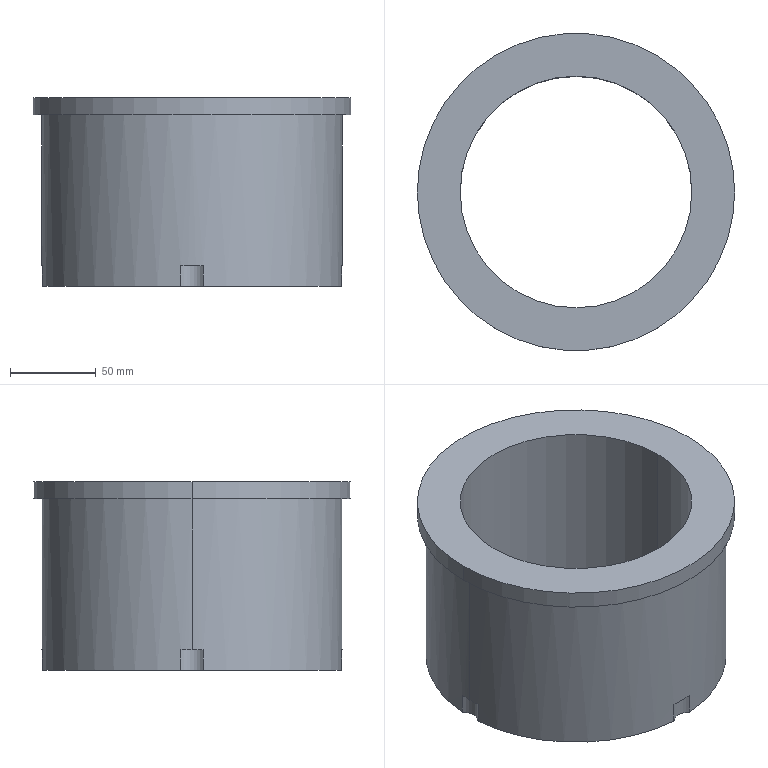Part | SolidWorks | features ICE 5, HoleWzd 1, Revolution 1 | 1 solid | 18 faces | box 185 x 185 x 110 mm | volume 1098272 mm3 | cylinder 11 | plane 7 | commonest cylinder face diameters 18 x5 135 x2 175 x2 185 x2
STEP:
#1=CARTESIAN_POINT('',(453.731,234.744,-1357.693));
#2=VERTEX_POINT('',#1);
#3=CARTESIAN_POINT('',(588.731,234.744,-1357.693));
#4=VERTEX_POINT('',#3);
#5=CARTESIAN_POINT('',(521.231,234.744,-1357.693));
#6=DIRECTION('',(0.,0.,1.));
#7=DIRECTION('',(1.,0.,0.));
#8=AXIS2_PLACEMENT_3D('',#5,#6,#7);
#9=CIRCLE('',#8,67.5);
#10=EDGE_CURVE('',#2,#4,#9,.T.);
#11=ORIENTED_EDGE('',*,*,#10,.F.);
#12=CARTESIAN_POINT('',(453.731,234.744,-1247.693));
#13=VERTEX_POINT('',#12);
#14=CARTESIAN_POINT('',(453.731,234.744,-1247.693));
#15=DIRECTION('',(0.,0.,1.));
#16=VECTOR('',#15,1000.);
#17=LINE('',#14,#16);
#18=EDGE_CURVE('',#2,#13,#17,.T.);
#19=ORIENTED_EDGE('',*,*,#18,.T.);
#20=CARTESIAN_POINT('',(588.731,234.744,-1247.693));
#21=VERTEX_POINT('',#20);
#22=CARTESIAN_POINT('',(521.231,234.744,-1247.693));
#23=DIRECTION('',(0.,0.,1.));
#24=DIRECTION('',(1.,0.,0.));
#25=AXIS2_PLACEMENT_3D('',#22,#23,#24);
#26=CIRCLE('',#25,67.5);
#27=EDGE_CURVE('',#13,#21,#26,.T.);
#28=ORIENTED_EDGE('',*,*,#27,.T.);
#29=CARTESIAN_POINT('',(588.731,234.744,-1247.693));
#30=DIRECTION('',(0.,0.,1.));
#31=VECTOR('',#30,1000.);
#32=LINE('',#29,#31);
#33=EDGE_CURVE('',#4,#21,#32,.T.);
#34=ORIENTED_EDGE('',*,*,#33,.F.);
#35=EDGE_LOOP('',(#11,#19,#28,#34));
#36=FACE_OUTER_BOUND('',#35,.T.);
#37=CARTESIAN_POINT('',(521.231,234.744,-1247.693));
#38=DIRECTION('',(0.,0.,1.));
#39=DIRECTION('',(1.,0.,0.));
#40=AXIS2_PLACEMENT_3D('',#37,#38,#39);
#41=CYLINDRICAL_SURFACE('',#40,67.5);
#42=ADVANCED_FACE('',(#36),#41,.F.);
#43=CARTESIAN_POINT('',(605.731,234.744,-1345.693));
#44=VERTEX_POINT('',#43);
#45=CARTESIAN_POINT('',(608.49,241.229,-1345.693));
#46=VERTEX_POINT('',#45);
#47=CARTESIAN_POINT('',(614.731,234.744,-1345.693));
#48=DIRECTION('',(0.,0.,-1.));
#49=DIRECTION('',(-1.,0.,0.));
#50=AXIS2_PLACEMENT_3D('',#47,#48,#49);
#51=CIRCLE('',#50,9.);
#52=EDGE_CURVE('',#44,#46,#51,.T.);
#53=ORIENTED_EDGE('',*,*,#52,.F.);
#54=CARTESIAN_POINT('',(605.731,234.744,-1357.693));
#55=VERTEX_POINT('',#54);
#56=CARTESIAN_POINT('',(605.731,234.744,-1345.693));
#57=DIRECTION('',(0.,0.,-1.));
#58=VECTOR('',#57,1000.);
#59=LINE('',#56,#58);
#60=EDGE_CURVE('',#44,#55,#59,.T.);
#61=ORIENTED_EDGE('',*,*,#60,.T.);
#62=CARTESIAN_POINT('',(608.49,241.229,-1357.693));
#63=VERTEX_POINT('',#62);
#64=CARTESIAN_POINT('',(614.731,234.744,-1357.693));
#65=DIRECTION('',(0.,0.,-1.));
#66=DIRECTION('',(-1.,0.,0.));
#67=AXIS2_PLACEMENT_3D('',#64,#65,#66);
#68=CIRCLE('',#67,9.);
#69=EDGE_CURVE('',#55,#63,#68,.T.);
#70=ORIENTED_EDGE('',*,*,#69,.T.);
#71=CARTESIAN_POINT('',(608.49,241.229,-1345.693));
#72=DIRECTION('',(0.,0.,-1.));
#73=VECTOR('',#72,1000.);
#74=LINE('',#71,#73);
#75=EDGE_CURVE('',#46,#63,#74,.T.);
#76=ORIENTED_EDGE('',*,*,#75,.F.);
#77=EDGE_LOOP('',(#53,#61,#70,#76));
#78=FACE_OUTER_BOUND('',#77,.T.);
#79=CARTESIAN_POINT('',(614.731,234.744,-1345.693));
#80=DIRECTION('',(0.,0.,-1.));
#81=DIRECTION('',(-1.,0.,0.));
#82=AXIS2_PLACEMENT_3D('',#79,#80,#81);
#83=CYLINDRICAL_SURFACE('',#82,9.);
#84=ADVANCED_FACE('',(#78),#83,.F.);
#85=CARTESIAN_POINT('',(433.731,234.744,-1345.693));
#86=VERTEX_POINT('',#85);
#87=CARTESIAN_POINT('',(433.971,241.229,-1345.693));
#88=VERTEX_POINT('',#87);
#89=CARTESIAN_POINT('',(521.231,234.744,-1345.693));
#90=DIRECTION('',(0.,0.,-1.));
#91=DIRECTION('',(-1.,0.,0.));
#92=AXIS2_PLACEMENT_3D('',#89,#90,#91);
#93=CIRCLE('',#92,87.5);
#94=EDGE_CURVE('',#86,#88,#93,.T.);
#95=ORIENTED_EDGE('',*,*,#94,.F.);
#96=CARTESIAN_POINT('',(433.731,234.744,-1257.693));
#97=VERTEX_POINT('',#96);
#98=CARTESIAN_POINT('',(433.731,234.744,-1357.693));
#99=DIRECTION('',(0.,0.,1.));
#100=VECTOR('',#99,1000.);
#101=LINE('',#98,#100);
#102=EDGE_CURVE('',#86,#97,#101,.T.);
#103=ORIENTED_EDGE('',*,*,#102,.T.);
#104=CARTESIAN_POINT('',(608.731,234.744,-1257.693));
#105=VERTEX_POINT('',#104);
#106=CARTESIAN_POINT('',(521.231,234.744,-1257.693));
#107=DIRECTION('',(0.,0.,-1.));
#108=DIRECTION('',(-1.,0.,0.));
#109=AXIS2_PLACEMENT_3D('',#106,#107,#108);
#110=CIRCLE('',#109,87.5);
#111=EDGE_CURVE('',#97,#105,#110,.T.);
#112=ORIENTED_EDGE('',*,*,#111,.T.);
#113=CARTESIAN_POINT('',(608.731,234.744,-1345.693));
#114=VERTEX_POINT('',#113);
#115=CARTESIAN_POINT('',(608.731,234.744,-1357.693));
#116=DIRECTION('',(0.,0.,1.));
#117=VECTOR('',#116,1000.);
#118=LINE('',#115,#117);
#119=EDGE_CURVE('',#114,#105,#118,.T.);
#120=ORIENTED_EDGE('',*,*,#119,.F.);
#121=CARTESIAN_POINT('',(521.231,234.744,-1345.693));
#122=DIRECTION('',(0.,0.,-1.));
#123=DIRECTION('',(-1.,0.,0.));
#124=AXIS2_PLACEMENT_3D('',#121,#122,#123);
#125=CIRCLE('',#124,87.5);
#126=EDGE_CURVE('',#46,#114,#125,.T.);
#127=ORIENTED_EDGE('',*,*,#126,.F.);
#128=ORIENTED_EDGE('',*,*,#75,.T.);
#129=CARTESIAN_POINT('',(527.716,322.003,-1357.693));
#130=VERTEX_POINT('',#129);
#131=CARTESIAN_POINT('',(521.231,234.744,-1357.693));
#132=DIRECTION('',(0.,0.,-1.));
#133=DIRECTION('',(-1.,0.,0.));
#134=AXIS2_PLACEMENT_3D('',#131,#132,#133);
#135=CIRCLE('',#134,87.5);
#136=EDGE_CURVE('',#130,#63,#135,.T.);
#137=ORIENTED_EDGE('',*,*,#136,.F.);
#138=CARTESIAN_POINT('',(527.716,322.003,-1345.693));
#139=VERTEX_POINT('',#138);
#140=CARTESIAN_POINT('',(527.716,322.003,-1345.693));
#141=DIRECTION('',(0.,0.,-1.));
#142=VECTOR('',#141,1000.);
#143=LINE('',#140,#142);
#144=EDGE_CURVE('',#139,#130,#143,.T.);
#145=ORIENTED_EDGE('',*,*,#144,.F.);
#146=CARTESIAN_POINT('',(514.746,322.003,-1345.693));
#147=VERTEX_POINT('',#146);
#148=CARTESIAN_POINT('',(521.231,234.744,-1345.693));
#149=DIRECTION('',(0.,0.,-1.));
#150=DIRECTION('',(-1.,0.,0.));
#151=AXIS2_PLACEMENT_3D('',#148,#149,#150);
#152=CIRCLE('',#151,87.5);
#153=EDGE_CURVE('',#147,#139,#152,.T.);
#154=ORIENTED_EDGE('',*,*,#153,.F.);
#155=CARTESIAN_POINT('',(514.746,322.003,-1357.693));
#156=VERTEX_POINT('',#155);
#157=CARTESIAN_POINT('',(514.746,322.003,-1345.693));
#158=DIRECTION('',(0.,0.,-1.));
#159=VECTOR('',#158,1000.);
#160=LINE('',#157,#159);
#161=EDGE_CURVE('',#147,#156,#160,.T.);
#162=ORIENTED_EDGE('',*,*,#161,.T.);
#163=CARTESIAN_POINT('',(433.971,241.229,-1357.693));
#164=VERTEX_POINT('',#163);
#165=CARTESIAN_POINT('',(521.231,234.744,-1357.693));
#166=DIRECTION('',(0.,0.,-1.));
#167=DIRECTION('',(-1.,0.,0.));
#168=AXIS2_PLACEMENT_3D('',#165,#166,#167);
#169=CIRCLE('',#168,87.5);
#170=EDGE_CURVE('',#164,#156,#169,.T.);
#171=ORIENTED_EDGE('',*,*,#170,.F.);
#172=CARTESIAN_POINT('',(433.971,241.229,-1345.693));
#173=DIRECTION('',(0.,0.,-1.));
#174=VECTOR('',#173,1000.);
#175=LINE('',#172,#174);
#176=EDGE_CURVE('',#88,#164,#175,.T.);
#177=ORIENTED_EDGE('',*,*,#176,.F.);
#178=EDGE_LOOP('',(#95,#103,#112,#120,#127,#128,#137,#145,#154,#162,#171,#177));
#179=FACE_OUTER_BOUND('',#178,.T.);
#180=CARTESIAN_POINT('',(521.231,234.744,-1357.693));
#181=DIRECTION('',(0.,0.,1.));
#182=DIRECTION('',(1.,0.,0.));
#183=AXIS2_PLACEMENT_3D('',#180,#181,#182);
#184=CYLINDRICAL_SURFACE('',#183,87.5);
#185=ADVANCED_FACE('',(#179),#184,.T.);
#186=CARTESIAN_POINT('',(613.731,234.744,-1257.693));
#187=VERTEX_POINT('',#186);
#188=CARTESIAN_POINT('',(428.731,234.744,-1257.693));
#189=VERTEX_POINT('',#188);
#190=CARTESIAN_POINT('',(521.231,234.744,-1257.693));
#191=DIRECTION('',(0.,0.,1.));
#192=DIRECTION('',(1.,0.,0.));
#193=AXIS2_PLACEMENT_3D('',#190,#191,#192);
#194=CIRCLE('',#193,92.5);
#195=EDGE_CURVE('',#187,#189,#194,.T.);
#196=ORIENTED_EDGE('',*,*,#195,.T.);
#197=CARTESIAN_POINT('',(428.731,234.744,-1247.693));
#198=VERTEX_POINT('',#197);
#199=CARTESIAN_POINT('',(428.731,234.744,-1257.693));
#200=DIRECTION('',(0.,0.,1.));
#201=VECTOR('',#200,1000.);
#202=LINE('',#199,#201);
#203=EDGE_CURVE('',#189,#198,#202,.T.);
#204=ORIENTED_EDGE('',*,*,#203,.T.);
#205=CARTESIAN_POINT('',(613.731,234.744,-1247.693));
#206=VERTEX_POINT('',#205);
#207=CARTESIAN_POINT('',(521.231,234.744,-1247.693));
#208=DIRECTION('',(0.,0.,1.));
#209=DIRECTION('',(1.,0.,0.));
#210=AXIS2_PLACEMENT_3D('',#207,#208,#209);
#211=CIRCLE('',#210,92.5);
#212=EDGE_CURVE('',#206,#198,#211,.T.);
#213=ORIENTED_EDGE('',*,*,#212,.F.);
#214=CARTESIAN_POINT('',(613.731,234.744,-1257.693));
#215=DIRECTION('',(0.,0.,1.));
#216=VECTOR('',#215,1000.);
#217=LINE('',#214,#216);
#218=EDGE_CURVE('',#187,#206,#217,.T.);
#219=ORIENTED_EDGE('',*,*,#218,.F.);
#220=EDGE_LOOP('',(#196,#204,#213,#219));
#221=FACE_OUTER_BOUND('',#220,.T.);
#222=CARTESIAN_POINT('',(521.231,234.744,-1257.693));
#223=DIRECTION('',(0.,0.,1.));
#224=DIRECTION('',(1.,0.,0.));
#225=AXIS2_PLACEMENT_3D('',#222,#223,#224);
#226=CYLINDRICAL_SURFACE('',#225,92.5);
#227=ADVANCED_FACE('',(#221),#226,.T.);
#228=CARTESIAN_POINT('',(608.49,228.259,-1357.693));
#229=VERTEX_POINT('',#228);
#230=CARTESIAN_POINT('',(614.731,234.744,-1357.693));
#231=DIRECTION('',(0.,0.,-1.));
#232=DIRECTION('',(-1.,0.,0.));
#233=AXIS2_PLACEMENT_3D('',#230,#231,#232);
#234=CIRCLE('',#233,9.);
#235=EDGE_CURVE('',#229,#55,#234,.T.);
#236=ORIENTED_EDGE('',*,*,#235,.F.);
#237=CARTESIAN_POINT('',(527.716,147.485,-1357.693));
#238=VERTEX_POINT('',#237);
#239=CARTESIAN_POINT('',(521.231,234.744,-1357.693));
#240=DIRECTION('',(0.,0.,-1.));
#241=DIRECTION('',(-1.,0.,0.));
#242=AXIS2_PLACEMENT_3D('',#239,#240,#241);
#243=CIRCLE('',#242,87.5);
#244=EDGE_CURVE('',#229,#238,#243,.T.);
#245=ORIENTED_EDGE('',*,*,#244,.T.);
#246=CARTESIAN_POINT('',(514.746,147.485,-1357.693));
#247=VERTEX_POINT('',#246);
#248=CARTESIAN_POINT('',(521.231,141.244,-1357.693));
#249=DIRECTION('',(0.,0.,-1.));
#250=DIRECTION('',(-1.,0.,0.));
#251=AXIS2_PLACEMENT_3D('',#248,#249,#250);
#252=CIRCLE('',#251,9.);
#253=EDGE_CURVE('',#247,#238,#252,.T.);
#254=ORIENTED_EDGE('',*,*,#253,.F.);
#255=CARTESIAN_POINT('',(433.971,228.259,-1357.693));
#256=VERTEX_POINT('',#255);
#257=CARTESIAN_POINT('',(521.231,234.744,-1357.693));
#258=DIRECTION('',(0.,0.,-1.));
#259=DIRECTION('',(-1.,0.,0.));
#260=AXIS2_PLACEMENT_3D('',#257,#258,#259);
#261=CIRCLE('',#260,87.5);
#262=EDGE_CURVE('',#247,#256,#261,.T.);
#263=ORIENTED_EDGE('',*,*,#262,.T.);
#264=CARTESIAN_POINT('',(427.731,234.744,-1357.693));
#265=DIRECTION('',(0.,0.,-1.));
#266=DIRECTION('',(-1.,0.,0.));
#267=AXIS2_PLACEMENT_3D('',#264,#265,#266);
#268=CIRCLE('',#267,9.);
#269=EDGE_CURVE('',#164,#256,#268,.T.);
#270=ORIENTED_EDGE('',*,*,#269,.F.);
#271=ORIENTED_EDGE('',*,*,#170,.T.);
#272=CARTESIAN_POINT('',(521.231,328.244,-1357.693));
#273=DIRECTION('',(0.,0.,-1.));
#274=DIRECTION('',(-1.,0.,0.));
#275=AXIS2_PLACEMENT_3D('',#272,#273,#274);
#276=CIRCLE('',#275,9.);
#277=EDGE_CURVE('',#130,#156,#276,.T.);
#278=ORIENTED_EDGE('',*,*,#277,.F.);
#279=ORIENTED_EDGE('',*,*,#136,.T.);
#280=ORIENTED_EDGE('',*,*,#69,.F.);
#281=EDGE_LOOP('',(#236,#245,#254,#263,#270,#271,#278,#279,#280));
#282=FACE_OUTER_BOUND('',#281,.T.);
#283=CARTESIAN_POINT('',(521.231,234.744,-1357.693));
#284=DIRECTION('',(0.,0.,1.));
#285=DIRECTION('',(1.,0.,0.));
#286=AXIS2_PLACEMENT_3D('',#283,#284,#285);
#287=CIRCLE('',#286,67.5);
#288=EDGE_CURVE('',#4,#2,#287,.T.);
#289=ORIENTED_EDGE('',*,*,#288,.T.);
#290=ORIENTED_EDGE('',*,*,#10,.T.);
#291=EDGE_LOOP('',(#289,#290));
#292=FACE_BOUND('',#291,.T.);
#293=CARTESIAN_POINT('',(521.231,234.744,-1357.693));
#294=DIRECTION('',(0.,0.,-1.));
#295=DIRECTION('',(-1.,0.,0.));
#296=AXIS2_PLACEMENT_3D('',#293,#294,#295);
#297=PLANE('',#296);
#298=ADVANCED_FACE('',(#282,#292),#297,.T.);
#299=ORIENTED_EDGE('',*,*,#203,.F.);
#300=CARTESIAN_POINT('',(521.231,234.744,-1257.693));
#301=DIRECTION('',(0.,0.,1.));
#302=DIRECTION('',(1.,0.,0.));
#303=AXIS2_PLACEMENT_3D('',#300,#301,#302);
#304=CIRCLE('',#303,92.5);
#305=EDGE_CURVE('',#189,#187,#304,.T.);
#306=ORIENTED_EDGE('',*,*,#305,.T.);
#307=ORIENTED_EDGE('',*,*,#218,.T.);
#308=CARTESIAN_POINT('',(521.231,234.744,-1247.693));
#309=DIRECTION('',(0.,0.,1.));
#310=DIRECTION('',(1.,0.,0.));
#311=AXIS2_PLACEMENT_3D('',#308,#309,#310);
#312=CIRCLE('',#311,92.5);
#313=EDGE_CURVE('',#198,#206,#312,.T.);
#314=ORIENTED_EDGE('',*,*,#313,.F.);
#315=EDGE_LOOP('',(#299,#306,#307,#314));
#316=FACE_OUTER_BOUND('',#315,.T.);
#317=CARTESIAN_POINT('',(521.231,234.744,-1257.693));
#318=DIRECTION('',(0.,0.,1.));
#319=DIRECTION('',(1.,0.,0.));
#320=AXIS2_PLACEMENT_3D('',#317,#318,#319);
#321=CYLINDRICAL_SURFACE('',#320,92.5);
#322=ADVANCED_FACE('',(#316),#321,.T.);
#323=CARTESIAN_POINT('',(521.231,234.744,-1257.693));
#324=DIRECTION('',(0.,0.,-1.));
#325=DIRECTION('',(-1.,0.,0.));
#326=AXIS2_PLACEMENT_3D('',#323,#324,#325);
#327=CIRCLE('',#326,87.5);
#328=EDGE_CURVE('',#105,#97,#327,.T.);
#329=ORIENTED_EDGE('',*,*,#328,.F.);
#330=ORIENTED_EDGE('',*,*,#111,.F.);
#331=EDGE_LOOP('',(#329,#330));
#332=FACE_BOUND('',#331,.T.);
#333=ORIENTED_EDGE('',*,*,#195,.F.);
#334=ORIENTED_EDGE('',*,*,#305,.F.);
#335=EDGE_LOOP('',(#333,#334));
#336=FACE_OUTER_BOUND('',#335,.T.);
#337=CARTESIAN_POINT('',(613.731,234.744,-1257.693));
#338=DIRECTION('',(0.,0.,-1.));
#339=DIRECTION('',(-1.,0.,0.));
#340=AXIS2_PLACEMENT_3D('',#337,#338,#339);
#341=PLANE('',#340);
#342=ADVANCED_FACE('',(#332,#336),#341,.T.);
#343=CARTESIAN_POINT('',(521.231,234.744,-1247.693));
#344=DIRECTION('',(0.,0.,1.));
#345=DIRECTION('',(1.,0.,0.));
#346=AXIS2_PLACEMENT_3D('',#343,#344,#345);
#347=CIRCLE('',#346,67.5);
#348=EDGE_CURVE('',#21,#13,#347,.T.);
#349=ORIENTED_EDGE('',*,*,#348,.F.);
#350=ORIENTED_EDGE('',*,*,#27,.F.);
#351=EDGE_LOOP('',(#349,#350));
#352=FACE_BOUND('',#351,.T.);
#353=ORIENTED_EDGE('',*,*,#212,.T.);
#354=ORIENTED_EDGE('',*,*,#313,.T.);
#355=EDGE_LOOP('',(#353,#354));
#356=FACE_OUTER_BOUND('',#355,.T.);
#357=CARTESIAN_POINT('',(521.231,234.744,-1247.693));
#358=DIRECTION('',(0.,0.,1.));
#359=DIRECTION('',(1.,0.,0.));
#360=AXIS2_PLACEMENT_3D('',#357,#358,#359);
#361=PLANE('',#360);
#362=ADVANCED_FACE('',(#352,#356),#361,.T.);
#363=ORIENTED_EDGE('',*,*,#102,.F.);
#364=CARTESIAN_POINT('',(433.971,228.259,-1345.693));
#365=VERTEX_POINT('',#364);
#366=CARTESIAN_POINT('',(521.231,234.744,-1345.693));
#367=DIRECTION('',(0.,0.,-1.));
#368=DIRECTION('',(-1.,0.,0.));
#369=AXIS2_PLACEMENT_3D('',#366,#367,#368);
#370=CIRCLE('',#369,87.5);
#371=EDGE_CURVE('',#365,#86,#370,.T.);
#372=ORIENTED_EDGE('',*,*,#371,.F.);
#373=CARTESIAN_POINT('',(433.971,228.259,-1345.693));
#374=DIRECTION('',(0.,0.,-1.));
#375=VECTOR('',#374,1000.);
#376=LINE('',#373,#375);
#377=EDGE_CURVE('',#365,#256,#376,.T.);
#378=ORIENTED_EDGE('',*,*,#377,.T.);
#379=ORIENTED_EDGE('',*,*,#262,.F.);
#380=CARTESIAN_POINT('',(514.746,147.485,-1345.693));
#381=VERTEX_POINT('',#380);
#382=CARTESIAN_POINT('',(514.746,147.485,-1345.693));
#383=DIRECTION('',(0.,0.,-1.));
#384=VECTOR('',#383,1000.);
#385=LINE('',#382,#384);
#386=EDGE_CURVE('',#381,#247,#385,.T.);
#387=ORIENTED_EDGE('',*,*,#386,.F.);
#388=CARTESIAN_POINT('',(527.716,147.485,-1345.693));
#389=VERTEX_POINT('',#388);
#390=CARTESIAN_POINT('',(521.231,234.744,-1345.693));
#391=DIRECTION('',(0.,0.,-1.));
#392=DIRECTION('',(-1.,0.,0.));
#393=AXIS2_PLACEMENT_3D('',#390,#391,#392);
#394=CIRCLE('',#393,87.5);
#395=EDGE_CURVE('',#389,#381,#394,.T.);
#396=ORIENTED_EDGE('',*,*,#395,.F.);
#397=CARTESIAN_POINT('',(527.716,147.485,-1345.693));
#398=DIRECTION('',(0.,0.,-1.));
#399=VECTOR('',#398,1000.);
#400=LINE('',#397,#399);
#401=EDGE_CURVE('',#389,#238,#400,.T.);
#402=ORIENTED_EDGE('',*,*,#401,.T.);
#403=ORIENTED_EDGE('',*,*,#244,.F.);
#404=CARTESIAN_POINT('',(608.49,228.259,-1345.693));
#405=VERTEX_POINT('',#404);
#406=CARTESIAN_POINT('',(608.49,228.259,-1345.693));
#407=DIRECTION('',(0.,0.,-1.));
#408=VECTOR('',#407,1000.);
#409=LINE('',#406,#408);
#410=EDGE_CURVE('',#405,#229,#409,.T.);
#411=ORIENTED_EDGE('',*,*,#410,.F.);
#412=CARTESIAN_POINT('',(521.231,234.744,-1345.693));
#413=DIRECTION('',(0.,0.,-1.));
#414=DIRECTION('',(-1.,0.,0.));
#415=AXIS2_PLACEMENT_3D('',#412,#413,#414);
#416=CIRCLE('',#415,87.5);
#417=EDGE_CURVE('',#114,#405,#416,.T.);
#418=ORIENTED_EDGE('',*,*,#417,.F.);
#419=ORIENTED_EDGE('',*,*,#119,.T.);
#420=ORIENTED_EDGE('',*,*,#328,.T.);
#421=EDGE_LOOP('',(#363,#372,#378,#379,#387,#396,#402,#403,#411,#418,#419,#420));
#422=FACE_OUTER_BOUND('',#421,.T.);
#423=CARTESIAN_POINT('',(521.231,234.744,-1357.693));
#424=DIRECTION('',(0.,0.,1.));
#425=DIRECTION('',(1.,0.,0.));
#426=AXIS2_PLACEMENT_3D('',#423,#424,#425);
#427=CYLINDRICAL_SURFACE('',#426,87.5);
#428=ADVANCED_FACE('',(#422),#427,.T.);
#429=ORIENTED_EDGE('',*,*,#269,.T.);
#430=ORIENTED_EDGE('',*,*,#377,.F.);
#431=CARTESIAN_POINT('',(427.731,234.744,-1345.693));
#432=DIRECTION('',(0.,0.,-1.));
#433=DIRECTION('',(-1.,0.,0.));
#434=AXIS2_PLACEMENT_3D('',#431,#432,#433);
#435=CIRCLE('',#434,9.);
#436=EDGE_CURVE('',#88,#365,#435,.T.);
#437=ORIENTED_EDGE('',*,*,#436,.F.);
#438=ORIENTED_EDGE('',*,*,#176,.T.);
#439=EDGE_LOOP('',(#429,#430,#437,#438));
#440=FACE_OUTER_BOUND('',#439,.T.);
#441=CARTESIAN_POINT('',(427.731,234.744,-1345.693));
#442=DIRECTION('',(0.,0.,-1.));
#443=DIRECTION('',(-1.,0.,0.));
#444=AXIS2_PLACEMENT_3D('',#441,#442,#443);
#445=CYLINDRICAL_SURFACE('',#444,9.);
#446=ADVANCED_FACE('',(#440),#445,.F.);
#447=ORIENTED_EDGE('',*,*,#371,.T.);
#448=ORIENTED_EDGE('',*,*,#94,.T.);
#449=ORIENTED_EDGE('',*,*,#436,.T.);
#450=EDGE_LOOP('',(#447,#448,#449));
#451=FACE_OUTER_BOUND('',#450,.T.);
#452=CARTESIAN_POINT('',(474.481,234.744,-1345.693));
#453=DIRECTION('',(0.,0.,-1.));
#454=DIRECTION('',(-1.,0.,0.));
#455=AXIS2_PLACEMENT_3D('',#452,#453,#454);
#456=PLANE('',#455);
#457=ADVANCED_FACE('',(#451),#456,.T.);
#458=ORIENTED_EDGE('',*,*,#253,.T.);
#459=ORIENTED_EDGE('',*,*,#401,.F.);
#460=CARTESIAN_POINT('',(521.231,141.244,-1345.693));
#461=DIRECTION('',(0.,0.,-1.));
#462=DIRECTION('',(-1.,0.,0.));
#463=AXIS2_PLACEMENT_3D('',#460,#461,#462);
#464=CIRCLE('',#463,9.);
#465=EDGE_CURVE('',#381,#389,#464,.T.);
#466=ORIENTED_EDGE('',*,*,#465,.F.);
#467=ORIENTED_EDGE('',*,*,#386,.T.);
#468=EDGE_LOOP('',(#458,#459,#466,#467));
#469=FACE_OUTER_BOUND('',#468,.T.);
#470=CARTESIAN_POINT('',(521.231,141.244,-1345.693));
#471=DIRECTION('',(0.,0.,-1.));
#472=DIRECTION('',(-1.,0.,0.));
#473=AXIS2_PLACEMENT_3D('',#470,#471,#472);
#474=CYLINDRICAL_SURFACE('',#473,9.);
#475=ADVANCED_FACE('',(#469),#474,.F.);
#476=ORIENTED_EDGE('',*,*,#395,.T.);
#477=ORIENTED_EDGE('',*,*,#465,.T.);
#478=EDGE_LOOP('',(#476,#477));
#479=FACE_OUTER_BOUND('',#478,.T.);
#480=CARTESIAN_POINT('',(521.231,187.994,-1345.693));
#481=DIRECTION('',(0.,0.,-1.));
#482=DIRECTION('',(-1.,0.,0.));
#483=AXIS2_PLACEMENT_3D('',#480,#481,#482);
#484=PLANE('',#483);
#485=ADVANCED_FACE('',(#479),#484,.T.);
#486=ORIENTED_EDGE('',*,*,#277,.T.);
#487=ORIENTED_EDGE('',*,*,#161,.F.);
#488=CARTESIAN_POINT('',(521.231,328.244,-1345.693));
#489=DIRECTION('',(0.,0.,-1.));
#490=DIRECTION('',(-1.,0.,0.));
#491=AXIS2_PLACEMENT_3D('',#488,#489,#490);
#492=CIRCLE('',#491,9.);
#493=EDGE_CURVE('',#139,#147,#492,.T.);
#494=ORIENTED_EDGE('',*,*,#493,.F.);
#495=ORIENTED_EDGE('',*,*,#144,.T.);
#496=EDGE_LOOP('',(#486,#487,#494,#495));
#497=FACE_OUTER_BOUND('',#496,.T.);
#498=CARTESIAN_POINT('',(521.231,328.244,-1345.693));
#499=DIRECTION('',(0.,0.,-1.));
#500=DIRECTION('',(-1.,0.,0.));
#501=AXIS2_PLACEMENT_3D('',#498,#499,#500);
#502=CYLINDRICAL_SURFACE('',#501,9.);
#503=ADVANCED_FACE('',(#497),#502,.F.);
#504=ORIENTED_EDGE('',*,*,#153,.T.);
#505=ORIENTED_EDGE('',*,*,#493,.T.);
#506=EDGE_LOOP('',(#504,#505));
#507=FACE_OUTER_BOUND('',#506,.T.);
#508=CARTESIAN_POINT('',(521.231,281.494,-1345.693));
#509=DIRECTION('',(0.,0.,-1.));
#510=DIRECTION('',(-1.,0.,0.));
#511=AXIS2_PLACEMENT_3D('',#508,#509,#510);
#512=PLANE('',#511);
#513=ADVANCED_FACE('',(#507),#512,.T.);
#514=ORIENTED_EDGE('',*,*,#60,.F.);
#515=CARTESIAN_POINT('',(614.731,234.744,-1345.693));
#516=DIRECTION('',(0.,0.,-1.));
#517=DIRECTION('',(-1.,0.,0.));
#518=AXIS2_PLACEMENT_3D('',#515,#516,#517);
#519=CIRCLE('',#518,9.);
#520=EDGE_CURVE('',#405,#44,#519,.T.);
#521=ORIENTED_EDGE('',*,*,#520,.F.);
#522=ORIENTED_EDGE('',*,*,#410,.T.);
#523=ORIENTED_EDGE('',*,*,#235,.T.);
#524=EDGE_LOOP('',(#514,#521,#522,#523));
#525=FACE_OUTER_BOUND('',#524,.T.);
#526=CARTESIAN_POINT('',(614.731,234.744,-1345.693));
#527=DIRECTION('',(0.,0.,-1.));
#528=DIRECTION('',(-1.,0.,0.));
#529=AXIS2_PLACEMENT_3D('',#526,#527,#528);
#530=CYLINDRICAL_SURFACE('',#529,9.);
#531=ADVANCED_FACE('',(#525),#530,.F.);
#532=ORIENTED_EDGE('',*,*,#126,.T.);
#533=ORIENTED_EDGE('',*,*,#417,.T.);
#534=ORIENTED_EDGE('',*,*,#520,.T.);
#535=ORIENTED_EDGE('',*,*,#52,.T.);
#536=EDGE_LOOP('',(#532,#533,#534,#535));
#537=FACE_OUTER_BOUND('',#536,.T.);
#538=CARTESIAN_POINT('',(567.981,234.744,-1345.693));
#539=DIRECTION('',(0.,0.,-1.));
#540=DIRECTION('',(-1.,0.,0.));
#541=AXIS2_PLACEMENT_3D('',#538,#539,#540);
#542=PLANE('',#541);
#543=ADVANCED_FACE('',(#537),#542,.T.);
#544=ORIENTED_EDGE('',*,*,#18,.F.);
#545=ORIENTED_EDGE('',*,*,#288,.F.);
#546=ORIENTED_EDGE('',*,*,#33,.T.);
#547=ORIENTED_EDGE('',*,*,#348,.T.);
#548=EDGE_LOOP('',(#544,#545,#546,#547));
#549=FACE_OUTER_BOUND('',#548,.T.);
#550=CARTESIAN_POINT('',(521.231,234.744,-1247.693));
#551=DIRECTION('',(0.,0.,1.));
#552=DIRECTION('',(1.,0.,0.));
#553=AXIS2_PLACEMENT_3D('',#550,#551,#552);
#554=CYLINDRICAL_SURFACE('',#553,67.5);
#555=ADVANCED_FACE('',(#549),#554,.F.);
#556=CLOSED_SHELL('',(#42,#84,#185,#227,#298,#322,#342,#362,#428,#446,#457,#475,#485,#503,#513,#531,#543,#555));
#557=MANIFOLD_SOLID_BREP('',#556);
#558=CARTESIAN_POINT('',(0.,0.,0.));
#559=DIRECTION('',(0.,0.,1.));
#560=DIRECTION('',(1.,0.,0.));
#561=AXIS2_PLACEMENT_3D('',#558,#559,#560);
#562=(LENGTH_UNIT()NAMED_UNIT(*)SI_UNIT(.MILLI.,.METRE.));
#563=UNCERTAINTY_MEASURE_WITH_UNIT(LENGTH_MEASURE(0.00001),#562,'','');
#564=(NAMED_UNIT(*)PLANE_ANGLE_UNIT()SI_UNIT($,.RADIAN.));
#565=(NAMED_UNIT(*)SI_UNIT($,.STERADIAN.)SOLID_ANGLE_UNIT());
#566=(GEOMETRIC_REPRESENTATION_CONTEXT(3)GLOBAL_UNCERTAINTY_ASSIGNED_CONTEXT((#563))GLOBAL_UNIT_ASSIGNED_CONTEXT((#562,#564,#565))REPRESENTATION_CONTEXT('',''));
#567=ADVANCED_BREP_SHAPE_REPRESENTATION('',(#557,#561),#566);